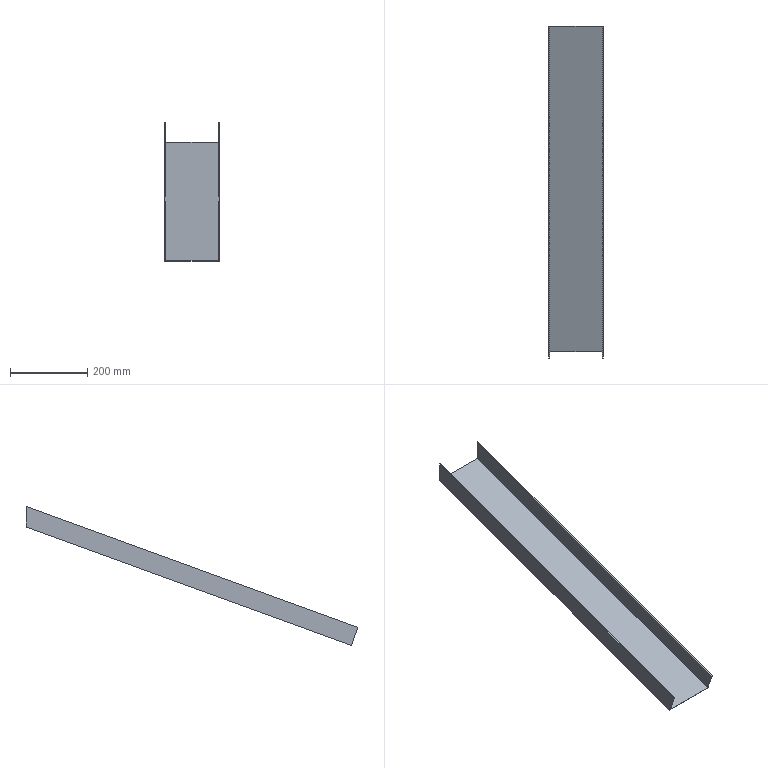Part | NX | features solid 2 | 1 solid | 10 faces | box 140 x 857.101 x 358.944 mm | volume 423844 mm3 | plane 10
STEP:
#1=CARTESIAN_POINT('',(-230.,-185.,-84.326));
#2=VERTEX_POINT('',#1);
#3=CARTESIAN_POINT('',(-228.,-185.,-84.326));
#4=VERTEX_POINT('',#3);
#5=CARTESIAN_POINT('',(-195.,-185.,-84.326));
#6=DIRECTION('',(1.,0.,0.));
#7=VECTOR('',#6,1000.);
#8=LINE('',#5,#7);
#9=EDGE_CURVE('',#2,#4,#8,.T.);
#10=ORIENTED_EDGE('',*,*,#9,.T.);
#11=CARTESIAN_POINT('',(-228.,-185.,-135.407));
#12=VERTEX_POINT('',#11);
#13=CARTESIAN_POINT('',(-228.,-185.,-215.937));
#14=DIRECTION('',(0.,0.,-1.));
#15=VECTOR('',#14,1000.);
#16=LINE('',#13,#15);
#17=EDGE_CURVE('',#4,#12,#16,.T.);
#18=ORIENTED_EDGE('',*,*,#17,.T.);
#19=CARTESIAN_POINT('',(-92.,-185.,-135.407));
#20=VERTEX_POINT('',#19);
#21=CARTESIAN_POINT('',(-195.,-185.,-135.407));
#22=DIRECTION('',(1.,0.,0.));
#23=VECTOR('',#22,1000.);
#24=LINE('',#21,#23);
#25=EDGE_CURVE('',#12,#20,#24,.T.);
#26=ORIENTED_EDGE('',*,*,#25,.T.);
#27=CARTESIAN_POINT('',(-92.,-185.,-84.326));
#28=VERTEX_POINT('',#27);
#29=CARTESIAN_POINT('',(-92.,-185.,40.));
#30=DIRECTION('',(0.,0.,-1.));
#31=VECTOR('',#30,1000.);
#32=LINE('',#29,#31);
#33=EDGE_CURVE('',#28,#20,#32,.T.);
#34=ORIENTED_EDGE('',*,*,#33,.F.);
#35=CARTESIAN_POINT('',(-90.,-185.,-84.326));
#36=VERTEX_POINT('',#35);
#37=CARTESIAN_POINT('',(-195.,-185.,-84.326));
#38=DIRECTION('',(1.,0.,0.));
#39=VECTOR('',#38,1000.);
#40=LINE('',#37,#39);
#41=EDGE_CURVE('',#28,#36,#40,.T.);
#42=ORIENTED_EDGE('',*,*,#41,.T.);
#43=CARTESIAN_POINT('',(-90.,-185.,-137.535));
#44=VERTEX_POINT('',#43);
#45=CARTESIAN_POINT('',(-90.,-185.,40.));
#46=DIRECTION('',(0.,0.,-1.));
#47=VECTOR('',#46,1000.);
#48=LINE('',#45,#47);
#49=EDGE_CURVE('',#36,#44,#48,.T.);
#50=ORIENTED_EDGE('',*,*,#49,.T.);
#51=CARTESIAN_POINT('',(-230.,-185.,-137.535));
#52=VERTEX_POINT('',#51);
#53=CARTESIAN_POINT('',(-195.,-185.,-137.535));
#54=DIRECTION('',(1.,0.,0.));
#55=VECTOR('',#54,1000.);
#56=LINE('',#53,#55);
#57=EDGE_CURVE('',#52,#44,#56,.T.);
#58=ORIENTED_EDGE('',*,*,#57,.F.);
#59=CARTESIAN_POINT('',(-230.,-185.,-215.937));
#60=DIRECTION('',(0.,0.,-1.));
#61=VECTOR('',#60,1000.);
#62=LINE('',#59,#61);
#63=EDGE_CURVE('',#2,#52,#62,.T.);
#64=ORIENTED_EDGE('',*,*,#63,.F.);
#65=EDGE_LOOP('',(#10,#18,#26,#34,#42,#50,#58,#64));
#66=FACE_BOUND('',#65,.T.);
#67=CARTESIAN_POINT('',(-1120.,-185.,40.));
#68=DIRECTION('',(0.,1.,0.));
#69=DIRECTION('',(-1.,0.,0.));
#70=AXIS2_PLACEMENT_3D('',#67,#68,#69);
#71=PLANE('',#70);
#72=ADVANCED_FACE('',(#66),#71,.T.);
#73=CARTESIAN_POINT('',(-90.,-1042.101,-396.286));
#74=VERTEX_POINT('',#73);
#75=CARTESIAN_POINT('',(-92.,-1042.101,-396.286));
#76=VERTEX_POINT('',#75);
#77=CARTESIAN_POINT('',(-195.,-1042.101,-396.286));
#78=DIRECTION('',(-1.,0.,0.));
#79=VECTOR('',#78,1000.);
#80=LINE('',#77,#79);
#81=EDGE_CURVE('',#74,#76,#80,.T.);
#82=ORIENTED_EDGE('',*,*,#81,.T.);
#83=CARTESIAN_POINT('',(-92.,-1025.684,-441.391));
#84=VERTEX_POINT('',#83);
#85=CARTESIAN_POINT('',(-92.,-1042.101,-396.286));
#86=DIRECTION('',(0.,0.342,-0.9397));
#87=VECTOR('',#86,1000.);
#88=LINE('',#85,#87);
#89=EDGE_CURVE('',#76,#84,#88,.T.);
#90=ORIENTED_EDGE('',*,*,#89,.T.);
#91=CARTESIAN_POINT('',(-228.,-1025.684,-441.391));
#92=VERTEX_POINT('',#91);
#93=CARTESIAN_POINT('',(-195.,-1025.684,-441.391));
#94=DIRECTION('',(-1.,0.,0.));
#95=VECTOR('',#94,1000.);
#96=LINE('',#93,#95);
#97=EDGE_CURVE('',#84,#92,#96,.T.);
#98=ORIENTED_EDGE('',*,*,#97,.T.);
#99=CARTESIAN_POINT('',(-228.,-1042.101,-396.286));
#100=VERTEX_POINT('',#99);
#101=CARTESIAN_POINT('',(-228.,-1042.101,-396.286));
#102=DIRECTION('',(0.,0.342,-0.9397));
#103=VECTOR('',#102,1000.);
#104=LINE('',#101,#103);
#105=EDGE_CURVE('',#100,#92,#104,.T.);
#106=ORIENTED_EDGE('',*,*,#105,.F.);
#107=CARTESIAN_POINT('',(-230.,-1042.101,-396.286));
#108=VERTEX_POINT('',#107);
#109=CARTESIAN_POINT('',(-195.,-1042.101,-396.286));
#110=DIRECTION('',(-1.,0.,0.));
#111=VECTOR('',#110,1000.);
#112=LINE('',#109,#111);
#113=EDGE_CURVE('',#100,#108,#112,.T.);
#114=ORIENTED_EDGE('',*,*,#113,.T.);
#115=CARTESIAN_POINT('',(-230.,-1025.,-443.27));
#116=VERTEX_POINT('',#115);
#117=CARTESIAN_POINT('',(-230.,-1042.101,-396.286));
#118=DIRECTION('',(0.,0.342,-0.9397));
#119=VECTOR('',#118,1000.);
#120=LINE('',#117,#119);
#121=EDGE_CURVE('',#108,#116,#120,.T.);
#122=ORIENTED_EDGE('',*,*,#121,.T.);
#123=CARTESIAN_POINT('',(-90.,-1025.,-443.27));
#124=VERTEX_POINT('',#123);
#125=CARTESIAN_POINT('',(-195.,-1025.,-443.27));
#126=DIRECTION('',(-1.,0.,0.));
#127=VECTOR('',#126,1000.);
#128=LINE('',#125,#127);
#129=EDGE_CURVE('',#124,#116,#128,.T.);
#130=ORIENTED_EDGE('',*,*,#129,.F.);
#131=CARTESIAN_POINT('',(-90.,-1042.101,-396.286));
#132=DIRECTION('',(0.,0.342,-0.9397));
#133=VECTOR('',#132,1000.);
#134=LINE('',#131,#133);
#135=EDGE_CURVE('',#74,#124,#134,.T.);
#136=ORIENTED_EDGE('',*,*,#135,.F.);
#137=EDGE_LOOP('',(#82,#90,#98,#106,#114,#122,#130,#136));
#138=FACE_BOUND('',#137,.T.);
#139=CARTESIAN_POINT('',(-195.,-1042.101,-396.286));
#140=DIRECTION('',(0.,-0.9397,-0.342));
#141=DIRECTION('',(0.,0.342,-0.9397));
#142=AXIS2_PLACEMENT_3D('',#139,#140,#141);
#143=PLANE('',#142);
#144=ADVANCED_FACE('',(#138),#143,.T.);
#145=ORIENTED_EDGE('',*,*,#113,.F.);
#146=CARTESIAN_POINT('',(-228.,-546.597,-215.937));
#147=DIRECTION('',(0.,0.9397,0.342));
#148=VECTOR('',#147,1000.);
#149=LINE('',#146,#148);
#150=EDGE_CURVE('',#100,#4,#149,.T.);
#151=ORIENTED_EDGE('',*,*,#150,.T.);
#152=ORIENTED_EDGE('',*,*,#9,.F.);
#153=CARTESIAN_POINT('',(-230.,-546.597,-215.937));
#154=DIRECTION('',(0.,0.9397,0.342));
#155=VECTOR('',#154,1000.);
#156=LINE('',#153,#155);
#157=EDGE_CURVE('',#108,#2,#156,.T.);
#158=ORIENTED_EDGE('',*,*,#157,.F.);
#159=EDGE_LOOP('',(#145,#151,#152,#158));
#160=FACE_BOUND('',#159,.T.);
#161=CARTESIAN_POINT('',(-195.,-546.597,-215.937));
#162=DIRECTION('',(0.,0.342,-0.9397));
#163=DIRECTION('',(-1.,0.,0.));
#164=AXIS2_PLACEMENT_3D('',#161,#162,#163);
#165=PLANE('',#164);
#166=ADVANCED_FACE('',(#160),#165,.F.);
#167=CARTESIAN_POINT('',(-230.,-529.496,-262.921));
#168=DIRECTION('',(0.,0.9397,0.342));
#169=VECTOR('',#168,1000.);
#170=LINE('',#167,#169);
#171=EDGE_CURVE('',#116,#52,#170,.T.);
#172=ORIENTED_EDGE('',*,*,#171,.F.);
#173=ORIENTED_EDGE('',*,*,#121,.F.);
#174=ORIENTED_EDGE('',*,*,#157,.T.);
#175=ORIENTED_EDGE('',*,*,#63,.T.);
#176=EDGE_LOOP('',(#172,#173,#174,#175));
#177=FACE_BOUND('',#176,.T.);
#178=CARTESIAN_POINT('',(-230.,-546.597,-215.937));
#179=DIRECTION('',(-1.,0.,0.));
#180=DIRECTION('',(0.,0.08716,0.9962));
#181=AXIS2_PLACEMENT_3D('',#178,#179,#180);
#182=PLANE('',#181);
#183=ADVANCED_FACE('',(#177),#182,.T.);
#184=CARTESIAN_POINT('',(-90.,-529.496,-262.921));
#185=DIRECTION('',(0.,-0.9397,-0.342));
#186=VECTOR('',#185,1000.);
#187=LINE('',#184,#186);
#188=EDGE_CURVE('',#44,#124,#187,.T.);
#189=ORIENTED_EDGE('',*,*,#188,.F.);
#190=ORIENTED_EDGE('',*,*,#49,.F.);
#191=CARTESIAN_POINT('',(-90.,-546.597,-215.937));
#192=DIRECTION('',(0.,-0.9397,-0.342));
#193=VECTOR('',#192,1000.);
#194=LINE('',#191,#193);
#195=EDGE_CURVE('',#36,#74,#194,.T.);
#196=ORIENTED_EDGE('',*,*,#195,.T.);
#197=ORIENTED_EDGE('',*,*,#135,.T.);
#198=EDGE_LOOP('',(#189,#190,#196,#197));
#199=FACE_BOUND('',#198,.T.);
#200=CARTESIAN_POINT('',(-90.,-546.597,-215.937));
#201=DIRECTION('',(1.,0.,0.));
#202=DIRECTION('',(0.,-0.08716,-0.9962));
#203=AXIS2_PLACEMENT_3D('',#200,#201,#202);
#204=PLANE('',#203);
#205=ADVANCED_FACE('',(#199),#204,.T.);
#206=ORIENTED_EDGE('',*,*,#41,.F.);
#207=CARTESIAN_POINT('',(-92.,-546.597,-215.937));
#208=DIRECTION('',(0.,-0.9397,-0.342));
#209=VECTOR('',#208,1000.);
#210=LINE('',#207,#209);
#211=EDGE_CURVE('',#28,#76,#210,.T.);
#212=ORIENTED_EDGE('',*,*,#211,.T.);
#213=ORIENTED_EDGE('',*,*,#81,.F.);
#214=ORIENTED_EDGE('',*,*,#195,.F.);
#215=EDGE_LOOP('',(#206,#212,#213,#214));
#216=FACE_BOUND('',#215,.T.);
#217=CARTESIAN_POINT('',(-195.,-546.597,-215.937));
#218=DIRECTION('',(0.,0.342,-0.9397));
#219=DIRECTION('',(-1.,0.,0.));
#220=AXIS2_PLACEMENT_3D('',#217,#218,#219);
#221=PLANE('',#220);
#222=ADVANCED_FACE('',(#216),#221,.F.);
#223=ORIENTED_EDGE('',*,*,#171,.T.);
#224=ORIENTED_EDGE('',*,*,#57,.T.);
#225=ORIENTED_EDGE('',*,*,#188,.T.);
#226=ORIENTED_EDGE('',*,*,#129,.T.);
#227=EDGE_LOOP('',(#223,#224,#225,#226));
#228=FACE_BOUND('',#227,.T.);
#229=CARTESIAN_POINT('',(-195.,-529.496,-262.921));
#230=DIRECTION('',(0.,0.342,-0.9397));
#231=DIRECTION('',(-1.,0.,0.));
#232=AXIS2_PLACEMENT_3D('',#229,#230,#231);
#233=PLANE('',#232);
#234=ADVANCED_FACE('',(#228),#233,.T.);
#235=CARTESIAN_POINT('',(-228.,-530.18,-261.042));
#236=DIRECTION('',(0.,0.9397,0.342));
#237=VECTOR('',#236,1000.);
#238=LINE('',#235,#237);
#239=EDGE_CURVE('',#92,#12,#238,.T.);
#240=ORIENTED_EDGE('',*,*,#239,.T.);
#241=ORIENTED_EDGE('',*,*,#17,.F.);
#242=ORIENTED_EDGE('',*,*,#150,.F.);
#243=ORIENTED_EDGE('',*,*,#105,.T.);
#244=EDGE_LOOP('',(#240,#241,#242,#243));
#245=FACE_BOUND('',#244,.T.);
#246=CARTESIAN_POINT('',(-228.,-546.597,-215.937));
#247=DIRECTION('',(-1.,0.,0.));
#248=DIRECTION('',(0.,0.08716,0.9962));
#249=AXIS2_PLACEMENT_3D('',#246,#247,#248);
#250=PLANE('',#249);
#251=ADVANCED_FACE('',(#245),#250,.F.);
#252=CARTESIAN_POINT('',(-92.,-530.18,-261.042));
#253=DIRECTION('',(0.,-0.9397,-0.342));
#254=VECTOR('',#253,1000.);
#255=LINE('',#252,#254);
#256=EDGE_CURVE('',#20,#84,#255,.T.);
#257=ORIENTED_EDGE('',*,*,#256,.T.);
#258=ORIENTED_EDGE('',*,*,#89,.F.);
#259=ORIENTED_EDGE('',*,*,#211,.F.);
#260=ORIENTED_EDGE('',*,*,#33,.T.);
#261=EDGE_LOOP('',(#257,#258,#259,#260));
#262=FACE_BOUND('',#261,.T.);
#263=CARTESIAN_POINT('',(-92.,-546.597,-215.937));
#264=DIRECTION('',(1.,0.,0.));
#265=DIRECTION('',(0.,-0.08716,-0.9962));
#266=AXIS2_PLACEMENT_3D('',#263,#264,#265);
#267=PLANE('',#266);
#268=ADVANCED_FACE('',(#262),#267,.F.);
#269=ORIENTED_EDGE('',*,*,#239,.F.);
#270=ORIENTED_EDGE('',*,*,#97,.F.);
#271=ORIENTED_EDGE('',*,*,#256,.F.);
#272=ORIENTED_EDGE('',*,*,#25,.F.);
#273=EDGE_LOOP('',(#269,#270,#271,#272));
#274=FACE_BOUND('',#273,.T.);
#275=CARTESIAN_POINT('',(-195.,-530.18,-261.042));
#276=DIRECTION('',(0.,0.342,-0.9397));
#277=DIRECTION('',(-1.,0.,0.));
#278=AXIS2_PLACEMENT_3D('',#275,#276,#277);
#279=PLANE('',#278);
#280=ADVANCED_FACE('',(#274),#279,.F.);
#281=CLOSED_SHELL('',(#72,#144,#166,#183,#205,#222,#234,#251,#268,#280));
#282=MANIFOLD_SOLID_BREP('',#281);
#283=(LENGTH_UNIT()NAMED_UNIT(*)SI_UNIT(.MILLI.,.METRE.));
#284=UNCERTAINTY_MEASURE_WITH_UNIT(LENGTH_MEASURE(0.00001),#283,'','');
#285=(NAMED_UNIT(*)PLANE_ANGLE_UNIT()SI_UNIT($,.RADIAN.));
#286=(NAMED_UNIT(*)SI_UNIT($,.STERADIAN.)SOLID_ANGLE_UNIT());
#287=(GEOMETRIC_REPRESENTATION_CONTEXT(3)GLOBAL_UNCERTAINTY_ASSIGNED_CONTEXT((#284))GLOBAL_UNIT_ASSIGNED_CONTEXT((#283,#285,#286))REPRESENTATION_CONTEXT('',''));
#288=ADVANCED_BREP_SHAPE_REPRESENTATION('',(#282),#287);